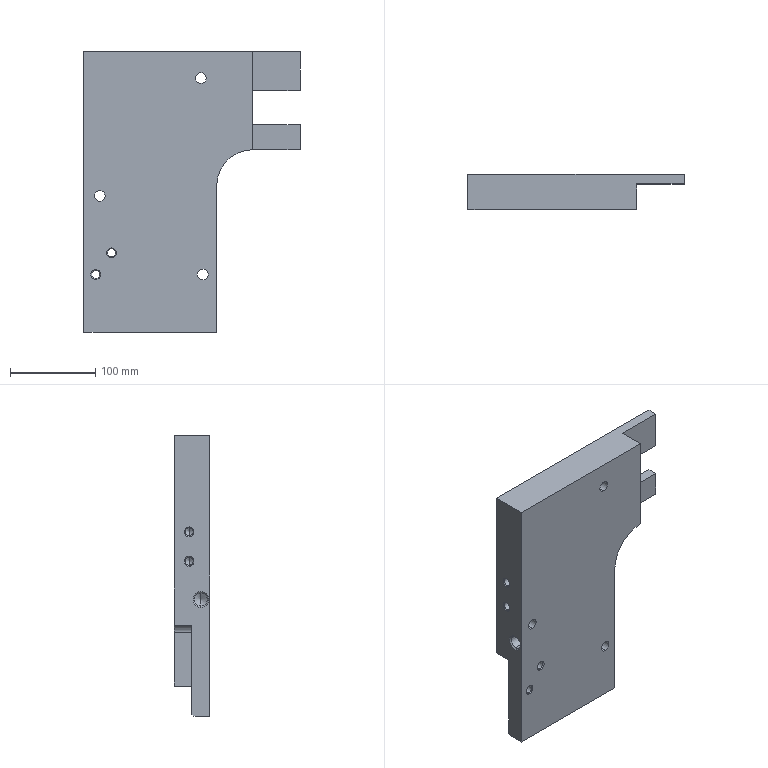Part | SolidWorks | features BaseBody 1 | 1 solid | 72 faces | box 253.846 x 41.538 x 330 mm | volume 1858895 mm3 | cylinder 27 | plane 25 | cone 20 | commonest cylinder face diameters 9.54 x8 12.692 x6 23.077 x6 15.339 x2 18.462 x1 40 x1